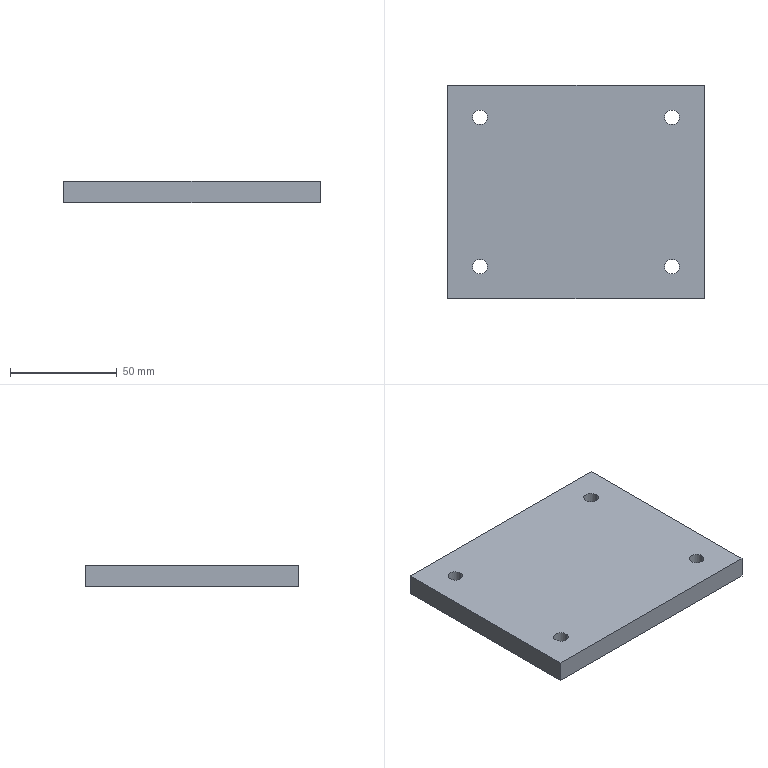Part | SolidWorks | features Extrusion 1, HoleWzd 1 | 1 solid | 14 faces | box 120 x 100 x 10 mm | volume 118547 mm3 | cylinder 8 | plane 6 | commonest cylinder face diameters 6.8 x8
STEP:
#1=CARTESIAN_POINT('',(48.4,-35.,0.));
#2=VERTEX_POINT('',#1);
#3=CARTESIAN_POINT('',(41.6,-35.,0.));
#4=VERTEX_POINT('',#3);
#5=CARTESIAN_POINT('',(45.,-35.,0.));
#6=DIRECTION('',(0.,0.,-1.));
#7=DIRECTION('',(-1.,0.,0.));
#8=AXIS2_PLACEMENT_3D('',#5,#6,#7);
#9=CIRCLE('',#8,3.4);
#10=EDGE_CURVE('',#2,#4,#9,.T.);
#11=ORIENTED_EDGE('',*,*,#10,.T.);
#12=CARTESIAN_POINT('',(41.6,-35.,10.));
#13=VERTEX_POINT('',#12);
#14=CARTESIAN_POINT('',(41.6,-35.,10.));
#15=DIRECTION('',(0.,0.,1.));
#16=VECTOR('',#15,1000.);
#17=LINE('',#14,#16);
#18=EDGE_CURVE('',#4,#13,#17,.T.);
#19=ORIENTED_EDGE('',*,*,#18,.T.);
#20=CARTESIAN_POINT('',(48.4,-35.,10.));
#21=VERTEX_POINT('',#20);
#22=CARTESIAN_POINT('',(45.,-35.,10.));
#23=DIRECTION('',(0.,0.,1.));
#24=DIRECTION('',(1.,0.,0.));
#25=AXIS2_PLACEMENT_3D('',#22,#23,#24);
#26=CIRCLE('',#25,3.4);
#27=EDGE_CURVE('',#13,#21,#26,.T.);
#28=ORIENTED_EDGE('',*,*,#27,.T.);
#29=CARTESIAN_POINT('',(48.4,-35.,10.));
#30=DIRECTION('',(0.,0.,1.));
#31=VECTOR('',#30,1000.);
#32=LINE('',#29,#31);
#33=EDGE_CURVE('',#2,#21,#32,.T.);
#34=ORIENTED_EDGE('',*,*,#33,.F.);
#35=EDGE_LOOP('',(#11,#19,#28,#34));
#36=FACE_OUTER_BOUND('',#35,.T.);
#37=CARTESIAN_POINT('',(45.,-35.,10.));
#38=DIRECTION('',(0.,0.,1.));
#39=DIRECTION('',(1.,0.,0.));
#40=AXIS2_PLACEMENT_3D('',#37,#38,#39);
#41=CYLINDRICAL_SURFACE('',#40,3.4);
#42=ADVANCED_FACE('',(#36),#41,.F.);
#43=CARTESIAN_POINT('',(-41.6,-35.,0.));
#44=VERTEX_POINT('',#43);
#45=CARTESIAN_POINT('',(-48.4,-35.,0.));
#46=VERTEX_POINT('',#45);
#47=CARTESIAN_POINT('',(-45.,-35.,0.));
#48=DIRECTION('',(0.,0.,-1.));
#49=DIRECTION('',(-1.,0.,0.));
#50=AXIS2_PLACEMENT_3D('',#47,#48,#49);
#51=CIRCLE('',#50,3.4);
#52=EDGE_CURVE('',#44,#46,#51,.T.);
#53=ORIENTED_EDGE('',*,*,#52,.T.);
#54=CARTESIAN_POINT('',(-48.4,-35.,10.));
#55=VERTEX_POINT('',#54);
#56=CARTESIAN_POINT('',(-48.4,-35.,10.));
#57=DIRECTION('',(0.,0.,1.));
#58=VECTOR('',#57,1000.);
#59=LINE('',#56,#58);
#60=EDGE_CURVE('',#46,#55,#59,.T.);
#61=ORIENTED_EDGE('',*,*,#60,.T.);
#62=CARTESIAN_POINT('',(-41.6,-35.,10.));
#63=VERTEX_POINT('',#62);
#64=CARTESIAN_POINT('',(-45.,-35.,10.));
#65=DIRECTION('',(0.,0.,1.));
#66=DIRECTION('',(1.,0.,0.));
#67=AXIS2_PLACEMENT_3D('',#64,#65,#66);
#68=CIRCLE('',#67,3.4);
#69=EDGE_CURVE('',#55,#63,#68,.T.);
#70=ORIENTED_EDGE('',*,*,#69,.T.);
#71=CARTESIAN_POINT('',(-41.6,-35.,10.));
#72=DIRECTION('',(0.,0.,1.));
#73=VECTOR('',#72,1000.);
#74=LINE('',#71,#73);
#75=EDGE_CURVE('',#44,#63,#74,.T.);
#76=ORIENTED_EDGE('',*,*,#75,.F.);
#77=EDGE_LOOP('',(#53,#61,#70,#76));
#78=FACE_OUTER_BOUND('',#77,.T.);
#79=CARTESIAN_POINT('',(-45.,-35.,10.));
#80=DIRECTION('',(0.,0.,1.));
#81=DIRECTION('',(1.,0.,0.));
#82=AXIS2_PLACEMENT_3D('',#79,#80,#81);
#83=CYLINDRICAL_SURFACE('',#82,3.4);
#84=ADVANCED_FACE('',(#78),#83,.F.);
#85=CARTESIAN_POINT('',(-41.6,35.,0.));
#86=VERTEX_POINT('',#85);
#87=CARTESIAN_POINT('',(-48.4,35.,0.));
#88=VERTEX_POINT('',#87);
#89=CARTESIAN_POINT('',(-45.,35.,0.));
#90=DIRECTION('',(0.,0.,-1.));
#91=DIRECTION('',(-1.,0.,0.));
#92=AXIS2_PLACEMENT_3D('',#89,#90,#91);
#93=CIRCLE('',#92,3.4);
#94=EDGE_CURVE('',#86,#88,#93,.T.);
#95=ORIENTED_EDGE('',*,*,#94,.T.);
#96=CARTESIAN_POINT('',(-48.4,35.,10.));
#97=VERTEX_POINT('',#96);
#98=CARTESIAN_POINT('',(-48.4,35.,10.));
#99=DIRECTION('',(0.,0.,1.));
#100=VECTOR('',#99,1000.);
#101=LINE('',#98,#100);
#102=EDGE_CURVE('',#88,#97,#101,.T.);
#103=ORIENTED_EDGE('',*,*,#102,.T.);
#104=CARTESIAN_POINT('',(-41.6,35.,10.));
#105=VERTEX_POINT('',#104);
#106=CARTESIAN_POINT('',(-45.,35.,10.));
#107=DIRECTION('',(0.,0.,1.));
#108=DIRECTION('',(1.,0.,0.));
#109=AXIS2_PLACEMENT_3D('',#106,#107,#108);
#110=CIRCLE('',#109,3.4);
#111=EDGE_CURVE('',#97,#105,#110,.T.);
#112=ORIENTED_EDGE('',*,*,#111,.T.);
#113=CARTESIAN_POINT('',(-41.6,35.,10.));
#114=DIRECTION('',(0.,0.,1.));
#115=VECTOR('',#114,1000.);
#116=LINE('',#113,#115);
#117=EDGE_CURVE('',#86,#105,#116,.T.);
#118=ORIENTED_EDGE('',*,*,#117,.F.);
#119=EDGE_LOOP('',(#95,#103,#112,#118));
#120=FACE_OUTER_BOUND('',#119,.T.);
#121=CARTESIAN_POINT('',(-45.,35.,10.));
#122=DIRECTION('',(0.,0.,1.));
#123=DIRECTION('',(1.,0.,0.));
#124=AXIS2_PLACEMENT_3D('',#121,#122,#123);
#125=CYLINDRICAL_SURFACE('',#124,3.4);
#126=ADVANCED_FACE('',(#120),#125,.F.);
#127=CARTESIAN_POINT('',(48.4,35.,0.));
#128=VERTEX_POINT('',#127);
#129=CARTESIAN_POINT('',(41.6,35.,0.));
#130=VERTEX_POINT('',#129);
#131=CARTESIAN_POINT('',(45.,35.,0.));
#132=DIRECTION('',(0.,0.,-1.));
#133=DIRECTION('',(-1.,0.,0.));
#134=AXIS2_PLACEMENT_3D('',#131,#132,#133);
#135=CIRCLE('',#134,3.4);
#136=EDGE_CURVE('',#128,#130,#135,.T.);
#137=ORIENTED_EDGE('',*,*,#136,.T.);
#138=CARTESIAN_POINT('',(41.6,35.,10.));
#139=VERTEX_POINT('',#138);
#140=CARTESIAN_POINT('',(41.6,35.,10.));
#141=DIRECTION('',(0.,0.,1.));
#142=VECTOR('',#141,1000.);
#143=LINE('',#140,#142);
#144=EDGE_CURVE('',#130,#139,#143,.T.);
#145=ORIENTED_EDGE('',*,*,#144,.T.);
#146=CARTESIAN_POINT('',(48.4,35.,10.));
#147=VERTEX_POINT('',#146);
#148=CARTESIAN_POINT('',(45.,35.,10.));
#149=DIRECTION('',(0.,0.,1.));
#150=DIRECTION('',(1.,0.,0.));
#151=AXIS2_PLACEMENT_3D('',#148,#149,#150);
#152=CIRCLE('',#151,3.4);
#153=EDGE_CURVE('',#139,#147,#152,.T.);
#154=ORIENTED_EDGE('',*,*,#153,.T.);
#155=CARTESIAN_POINT('',(48.4,35.,10.));
#156=DIRECTION('',(0.,0.,1.));
#157=VECTOR('',#156,1000.);
#158=LINE('',#155,#157);
#159=EDGE_CURVE('',#128,#147,#158,.T.);
#160=ORIENTED_EDGE('',*,*,#159,.F.);
#161=EDGE_LOOP('',(#137,#145,#154,#160));
#162=FACE_OUTER_BOUND('',#161,.T.);
#163=CARTESIAN_POINT('',(45.,35.,10.));
#164=DIRECTION('',(0.,0.,1.));
#165=DIRECTION('',(1.,0.,0.));
#166=AXIS2_PLACEMENT_3D('',#163,#164,#165);
#167=CYLINDRICAL_SURFACE('',#166,3.4);
#168=ADVANCED_FACE('',(#162),#167,.F.);
#169=CARTESIAN_POINT('',(-60.,50.,0.));
#170=VERTEX_POINT('',#169);
#171=CARTESIAN_POINT('',(-60.,-50.,0.));
#172=VERTEX_POINT('',#171);
#173=CARTESIAN_POINT('',(-60.,50.,0.));
#174=DIRECTION('',(0.,-1.,0.));
#175=VECTOR('',#174,1000.);
#176=LINE('',#173,#175);
#177=EDGE_CURVE('',#170,#172,#176,.T.);
#178=ORIENTED_EDGE('',*,*,#177,.T.);
#179=CARTESIAN_POINT('',(-60.,-50.,10.));
#180=VERTEX_POINT('',#179);
#181=CARTESIAN_POINT('',(-60.,-50.,10.));
#182=DIRECTION('',(0.,0.,-1.));
#183=VECTOR('',#182,1000.);
#184=LINE('',#181,#183);
#185=EDGE_CURVE('',#180,#172,#184,.T.);
#186=ORIENTED_EDGE('',*,*,#185,.F.);
#187=CARTESIAN_POINT('',(-60.,50.,10.));
#188=VERTEX_POINT('',#187);
#189=CARTESIAN_POINT('',(-60.,50.,10.));
#190=DIRECTION('',(0.,-1.,0.));
#191=VECTOR('',#190,1000.);
#192=LINE('',#189,#191);
#193=EDGE_CURVE('',#188,#180,#192,.T.);
#194=ORIENTED_EDGE('',*,*,#193,.F.);
#195=CARTESIAN_POINT('',(-60.,50.,10.));
#196=DIRECTION('',(0.,0.,-1.));
#197=VECTOR('',#196,1000.);
#198=LINE('',#195,#197);
#199=EDGE_CURVE('',#188,#170,#198,.T.);
#200=ORIENTED_EDGE('',*,*,#199,.T.);
#201=EDGE_LOOP('',(#178,#186,#194,#200));
#202=FACE_OUTER_BOUND('',#201,.T.);
#203=CARTESIAN_POINT('',(-60.,50.,10.));
#204=DIRECTION('',(1.,0.,0.));
#205=DIRECTION('',(0.,1.,0.));
#206=AXIS2_PLACEMENT_3D('',#203,#204,#205);
#207=PLANE('',#206);
#208=ADVANCED_FACE('',(#202),#207,.F.);
#209=CARTESIAN_POINT('',(60.,-50.,0.));
#210=VERTEX_POINT('',#209);
#211=CARTESIAN_POINT('',(60.,-50.,0.));
#212=DIRECTION('',(1.,0.,0.));
#213=VECTOR('',#212,1000.);
#214=LINE('',#211,#213);
#215=EDGE_CURVE('',#172,#210,#214,.T.);
#216=ORIENTED_EDGE('',*,*,#215,.T.);
#217=CARTESIAN_POINT('',(60.,-50.,10.));
#218=VERTEX_POINT('',#217);
#219=CARTESIAN_POINT('',(60.,-50.,10.));
#220=DIRECTION('',(0.,0.,-1.));
#221=VECTOR('',#220,1000.);
#222=LINE('',#219,#221);
#223=EDGE_CURVE('',#218,#210,#222,.T.);
#224=ORIENTED_EDGE('',*,*,#223,.F.);
#225=CARTESIAN_POINT('',(60.,-50.,10.));
#226=DIRECTION('',(1.,0.,0.));
#227=VECTOR('',#226,1000.);
#228=LINE('',#225,#227);
#229=EDGE_CURVE('',#180,#218,#228,.T.);
#230=ORIENTED_EDGE('',*,*,#229,.F.);
#231=ORIENTED_EDGE('',*,*,#185,.T.);
#232=EDGE_LOOP('',(#216,#224,#230,#231));
#233=FACE_OUTER_BOUND('',#232,.T.);
#234=CARTESIAN_POINT('',(60.,-50.,10.));
#235=DIRECTION('',(0.,1.,0.));
#236=DIRECTION('',(-1.,0.,0.));
#237=AXIS2_PLACEMENT_3D('',#234,#235,#236);
#238=PLANE('',#237);
#239=ADVANCED_FACE('',(#233),#238,.F.);
#240=CARTESIAN_POINT('',(60.,50.,0.));
#241=VERTEX_POINT('',#240);
#242=CARTESIAN_POINT('',(60.,50.,0.));
#243=DIRECTION('',(0.,1.,0.));
#244=VECTOR('',#243,1000.);
#245=LINE('',#242,#244);
#246=EDGE_CURVE('',#210,#241,#245,.T.);
#247=ORIENTED_EDGE('',*,*,#246,.T.);
#248=CARTESIAN_POINT('',(60.,50.,10.));
#249=VERTEX_POINT('',#248);
#250=CARTESIAN_POINT('',(60.,50.,10.));
#251=DIRECTION('',(0.,0.,-1.));
#252=VECTOR('',#251,1000.);
#253=LINE('',#250,#252);
#254=EDGE_CURVE('',#249,#241,#253,.T.);
#255=ORIENTED_EDGE('',*,*,#254,.F.);
#256=CARTESIAN_POINT('',(60.,50.,10.));
#257=DIRECTION('',(0.,1.,0.));
#258=VECTOR('',#257,1000.);
#259=LINE('',#256,#258);
#260=EDGE_CURVE('',#218,#249,#259,.T.);
#261=ORIENTED_EDGE('',*,*,#260,.F.);
#262=ORIENTED_EDGE('',*,*,#223,.T.);
#263=EDGE_LOOP('',(#247,#255,#261,#262));
#264=FACE_OUTER_BOUND('',#263,.T.);
#265=CARTESIAN_POINT('',(60.,50.,10.));
#266=DIRECTION('',(-1.,0.,0.));
#267=DIRECTION('',(0.,-1.,0.));
#268=AXIS2_PLACEMENT_3D('',#265,#266,#267);
#269=PLANE('',#268);
#270=ADVANCED_FACE('',(#264),#269,.F.);
#271=CARTESIAN_POINT('',(60.,50.,0.));
#272=DIRECTION('',(-1.,0.,0.));
#273=VECTOR('',#272,1000.);
#274=LINE('',#271,#273);
#275=EDGE_CURVE('',#241,#170,#274,.T.);
#276=ORIENTED_EDGE('',*,*,#275,.T.);
#277=ORIENTED_EDGE('',*,*,#199,.F.);
#278=CARTESIAN_POINT('',(60.,50.,10.));
#279=DIRECTION('',(-1.,0.,0.));
#280=VECTOR('',#279,1000.);
#281=LINE('',#278,#280);
#282=EDGE_CURVE('',#249,#188,#281,.T.);
#283=ORIENTED_EDGE('',*,*,#282,.F.);
#284=ORIENTED_EDGE('',*,*,#254,.T.);
#285=EDGE_LOOP('',(#276,#277,#283,#284));
#286=FACE_OUTER_BOUND('',#285,.T.);
#287=CARTESIAN_POINT('',(60.,50.,10.));
#288=DIRECTION('',(0.,-1.,0.));
#289=DIRECTION('',(1.,0.,0.));
#290=AXIS2_PLACEMENT_3D('',#287,#288,#289);
#291=PLANE('',#290);
#292=ADVANCED_FACE('',(#286),#291,.F.);
#293=CARTESIAN_POINT('',(45.,-35.,10.));
#294=DIRECTION('',(0.,0.,1.));
#295=DIRECTION('',(1.,0.,0.));
#296=AXIS2_PLACEMENT_3D('',#293,#294,#295);
#297=CIRCLE('',#296,3.4);
#298=EDGE_CURVE('',#21,#13,#297,.T.);
#299=ORIENTED_EDGE('',*,*,#298,.F.);
#300=ORIENTED_EDGE('',*,*,#27,.F.);
#301=EDGE_LOOP('',(#299,#300));
#302=FACE_BOUND('',#301,.T.);
#303=CARTESIAN_POINT('',(-45.,-35.,10.));
#304=DIRECTION('',(0.,0.,1.));
#305=DIRECTION('',(1.,0.,0.));
#306=AXIS2_PLACEMENT_3D('',#303,#304,#305);
#307=CIRCLE('',#306,3.4);
#308=EDGE_CURVE('',#63,#55,#307,.T.);
#309=ORIENTED_EDGE('',*,*,#308,.F.);
#310=ORIENTED_EDGE('',*,*,#69,.F.);
#311=EDGE_LOOP('',(#309,#310));
#312=FACE_BOUND('',#311,.T.);
#313=CARTESIAN_POINT('',(-45.,35.,10.));
#314=DIRECTION('',(0.,0.,1.));
#315=DIRECTION('',(1.,0.,0.));
#316=AXIS2_PLACEMENT_3D('',#313,#314,#315);
#317=CIRCLE('',#316,3.4);
#318=EDGE_CURVE('',#105,#97,#317,.T.);
#319=ORIENTED_EDGE('',*,*,#318,.F.);
#320=ORIENTED_EDGE('',*,*,#111,.F.);
#321=EDGE_LOOP('',(#319,#320));
#322=FACE_BOUND('',#321,.T.);
#323=CARTESIAN_POINT('',(45.,35.,10.));
#324=DIRECTION('',(0.,0.,1.));
#325=DIRECTION('',(1.,0.,0.));
#326=AXIS2_PLACEMENT_3D('',#323,#324,#325);
#327=CIRCLE('',#326,3.4);
#328=EDGE_CURVE('',#147,#139,#327,.T.);
#329=ORIENTED_EDGE('',*,*,#328,.F.);
#330=ORIENTED_EDGE('',*,*,#153,.F.);
#331=EDGE_LOOP('',(#329,#330));
#332=FACE_BOUND('',#331,.T.);
#333=ORIENTED_EDGE('',*,*,#193,.T.);
#334=ORIENTED_EDGE('',*,*,#229,.T.);
#335=ORIENTED_EDGE('',*,*,#260,.T.);
#336=ORIENTED_EDGE('',*,*,#282,.T.);
#337=EDGE_LOOP('',(#333,#334,#335,#336));
#338=FACE_OUTER_BOUND('',#337,.T.);
#339=CARTESIAN_POINT('',(0.,0.,10.));
#340=DIRECTION('',(0.,0.,-1.));
#341=DIRECTION('',(-1.,0.,0.));
#342=AXIS2_PLACEMENT_3D('',#339,#340,#341);
#343=PLANE('',#342);
#344=ADVANCED_FACE('',(#302,#312,#322,#332,#338),#343,.F.);
#345=ORIENTED_EDGE('',*,*,#10,.F.);
#346=CARTESIAN_POINT('',(45.,-35.,0.));
#347=DIRECTION('',(0.,0.,-1.));
#348=DIRECTION('',(-1.,0.,0.));
#349=AXIS2_PLACEMENT_3D('',#346,#347,#348);
#350=CIRCLE('',#349,3.4);
#351=EDGE_CURVE('',#4,#2,#350,.T.);
#352=ORIENTED_EDGE('',*,*,#351,.F.);
#353=EDGE_LOOP('',(#345,#352));
#354=FACE_BOUND('',#353,.T.);
#355=ORIENTED_EDGE('',*,*,#52,.F.);
#356=CARTESIAN_POINT('',(-45.,-35.,0.));
#357=DIRECTION('',(0.,0.,-1.));
#358=DIRECTION('',(-1.,0.,0.));
#359=AXIS2_PLACEMENT_3D('',#356,#357,#358);
#360=CIRCLE('',#359,3.4);
#361=EDGE_CURVE('',#46,#44,#360,.T.);
#362=ORIENTED_EDGE('',*,*,#361,.F.);
#363=EDGE_LOOP('',(#355,#362));
#364=FACE_BOUND('',#363,.T.);
#365=ORIENTED_EDGE('',*,*,#94,.F.);
#366=CARTESIAN_POINT('',(-45.,35.,0.));
#367=DIRECTION('',(0.,0.,-1.));
#368=DIRECTION('',(-1.,0.,0.));
#369=AXIS2_PLACEMENT_3D('',#366,#367,#368);
#370=CIRCLE('',#369,3.4);
#371=EDGE_CURVE('',#88,#86,#370,.T.);
#372=ORIENTED_EDGE('',*,*,#371,.F.);
#373=EDGE_LOOP('',(#365,#372));
#374=FACE_BOUND('',#373,.T.);
#375=ORIENTED_EDGE('',*,*,#136,.F.);
#376=CARTESIAN_POINT('',(45.,35.,0.));
#377=DIRECTION('',(0.,0.,-1.));
#378=DIRECTION('',(-1.,0.,0.));
#379=AXIS2_PLACEMENT_3D('',#376,#377,#378);
#380=CIRCLE('',#379,3.4);
#381=EDGE_CURVE('',#130,#128,#380,.T.);
#382=ORIENTED_EDGE('',*,*,#381,.F.);
#383=EDGE_LOOP('',(#375,#382));
#384=FACE_BOUND('',#383,.T.);
#385=ORIENTED_EDGE('',*,*,#177,.F.);
#386=ORIENTED_EDGE('',*,*,#275,.F.);
#387=ORIENTED_EDGE('',*,*,#246,.F.);
#388=ORIENTED_EDGE('',*,*,#215,.F.);
#389=EDGE_LOOP('',(#385,#386,#387,#388));
#390=FACE_OUTER_BOUND('',#389,.T.);
#391=CARTESIAN_POINT('',(0.,0.,0.));
#392=DIRECTION('',(0.,0.,-1.));
#393=DIRECTION('',(-1.,0.,0.));
#394=AXIS2_PLACEMENT_3D('',#391,#392,#393);
#395=PLANE('',#394);
#396=ADVANCED_FACE('',(#354,#364,#374,#384,#390),#395,.T.);
#397=ORIENTED_EDGE('',*,*,#144,.F.);
#398=ORIENTED_EDGE('',*,*,#381,.T.);
#399=ORIENTED_EDGE('',*,*,#159,.T.);
#400=ORIENTED_EDGE('',*,*,#328,.T.);
#401=EDGE_LOOP('',(#397,#398,#399,#400));
#402=FACE_OUTER_BOUND('',#401,.T.);
#403=CARTESIAN_POINT('',(45.,35.,10.));
#404=DIRECTION('',(0.,0.,1.));
#405=DIRECTION('',(1.,0.,0.));
#406=AXIS2_PLACEMENT_3D('',#403,#404,#405);
#407=CYLINDRICAL_SURFACE('',#406,3.4);
#408=ADVANCED_FACE('',(#402),#407,.F.);
#409=ORIENTED_EDGE('',*,*,#102,.F.);
#410=ORIENTED_EDGE('',*,*,#371,.T.);
#411=ORIENTED_EDGE('',*,*,#117,.T.);
#412=ORIENTED_EDGE('',*,*,#318,.T.);
#413=EDGE_LOOP('',(#409,#410,#411,#412));
#414=FACE_OUTER_BOUND('',#413,.T.);
#415=CARTESIAN_POINT('',(-45.,35.,10.));
#416=DIRECTION('',(0.,0.,1.));
#417=DIRECTION('',(1.,0.,0.));
#418=AXIS2_PLACEMENT_3D('',#415,#416,#417);
#419=CYLINDRICAL_SURFACE('',#418,3.4);
#420=ADVANCED_FACE('',(#414),#419,.F.);
#421=ORIENTED_EDGE('',*,*,#60,.F.);
#422=ORIENTED_EDGE('',*,*,#361,.T.);
#423=ORIENTED_EDGE('',*,*,#75,.T.);
#424=ORIENTED_EDGE('',*,*,#308,.T.);
#425=EDGE_LOOP('',(#421,#422,#423,#424));
#426=FACE_OUTER_BOUND('',#425,.T.);
#427=CARTESIAN_POINT('',(-45.,-35.,10.));
#428=DIRECTION('',(0.,0.,1.));
#429=DIRECTION('',(1.,0.,0.));
#430=AXIS2_PLACEMENT_3D('',#427,#428,#429);
#431=CYLINDRICAL_SURFACE('',#430,3.4);
#432=ADVANCED_FACE('',(#426),#431,.F.);
#433=ORIENTED_EDGE('',*,*,#18,.F.);
#434=ORIENTED_EDGE('',*,*,#351,.T.);
#435=ORIENTED_EDGE('',*,*,#33,.T.);
#436=ORIENTED_EDGE('',*,*,#298,.T.);
#437=EDGE_LOOP('',(#433,#434,#435,#436));
#438=FACE_OUTER_BOUND('',#437,.T.);
#439=CARTESIAN_POINT('',(45.,-35.,10.));
#440=DIRECTION('',(0.,0.,1.));
#441=DIRECTION('',(1.,0.,0.));
#442=AXIS2_PLACEMENT_3D('',#439,#440,#441);
#443=CYLINDRICAL_SURFACE('',#442,3.4);
#444=ADVANCED_FACE('',(#438),#443,.F.);
#445=CLOSED_SHELL('',(#42,#84,#126,#168,#208,#239,#270,#292,#344,#396,#408,#420,#432,#444));
#446=MANIFOLD_SOLID_BREP('',#445);
#447=CARTESIAN_POINT('',(0.,0.,0.));
#448=DIRECTION('',(0.,0.,1.));
#449=DIRECTION('',(1.,0.,0.));
#450=AXIS2_PLACEMENT_3D('',#447,#448,#449);
#451=(LENGTH_UNIT()NAMED_UNIT(*)SI_UNIT(.MILLI.,.METRE.));
#452=UNCERTAINTY_MEASURE_WITH_UNIT(LENGTH_MEASURE(0.00001),#451,'','');
#453=(NAMED_UNIT(*)PLANE_ANGLE_UNIT()SI_UNIT($,.RADIAN.));
#454=(NAMED_UNIT(*)SI_UNIT($,.STERADIAN.)SOLID_ANGLE_UNIT());
#455=(GEOMETRIC_REPRESENTATION_CONTEXT(3)GLOBAL_UNCERTAINTY_ASSIGNED_CONTEXT((#452))GLOBAL_UNIT_ASSIGNED_CONTEXT((#451,#453,#454))REPRESENTATION_CONTEXT('',''));
#456=ADVANCED_BREP_SHAPE_REPRESENTATION('',(#446,#450),#455);